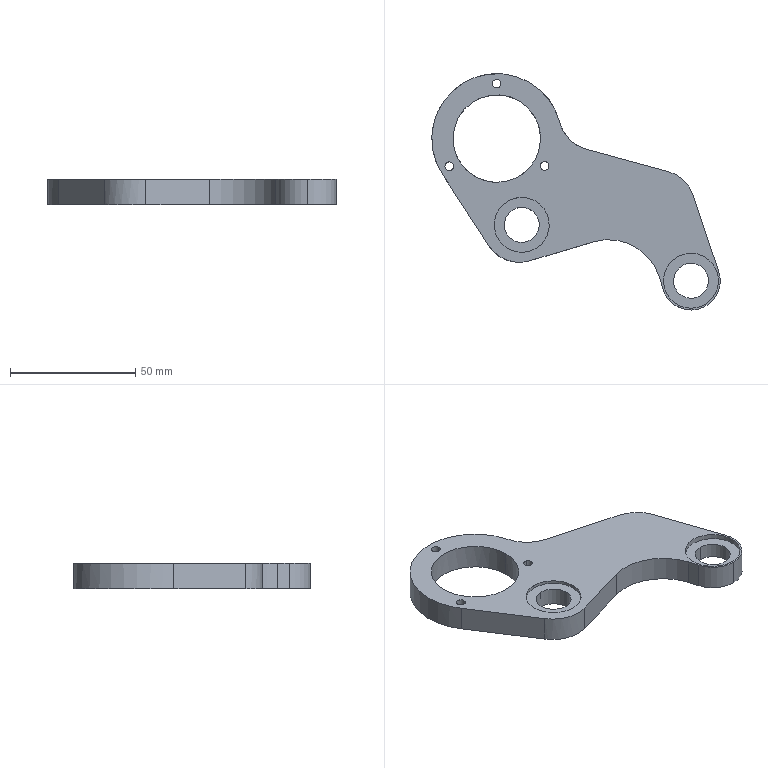Part | SolidWorks | features BaseBody 1 | 1 solid | 47 faces | box 115.387 x 94.571 x 10.017 mm | volume 39488 mm3 | cylinder 33 | plane 14 | commonest cylinder face diameters 22 x8 3.5 x6 7 x6 14 x4 23.4 x2 29.4 x2